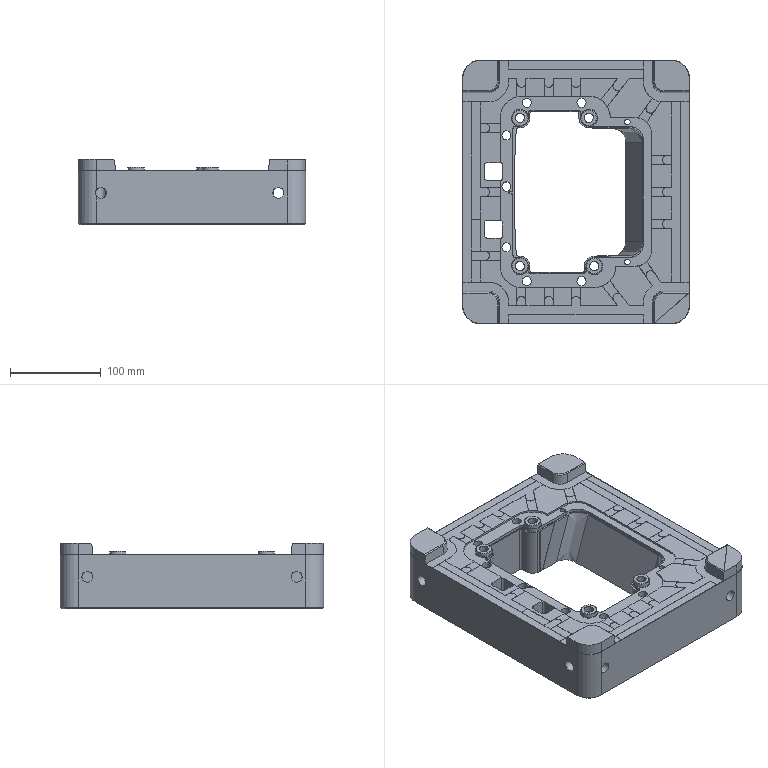Part | STEP file | solid 31 | 1 solid | 422 faces | box 250 x 290 x 72 mm | volume 2895131 mm3 | plane 176 | cylinder 112 | spline 61 | cone 33 | torus 25 | other 15 | commonest cylinder face diameters 10 x27 12 x23 0.602 x15 4 x8 6 x6 10.2 x6